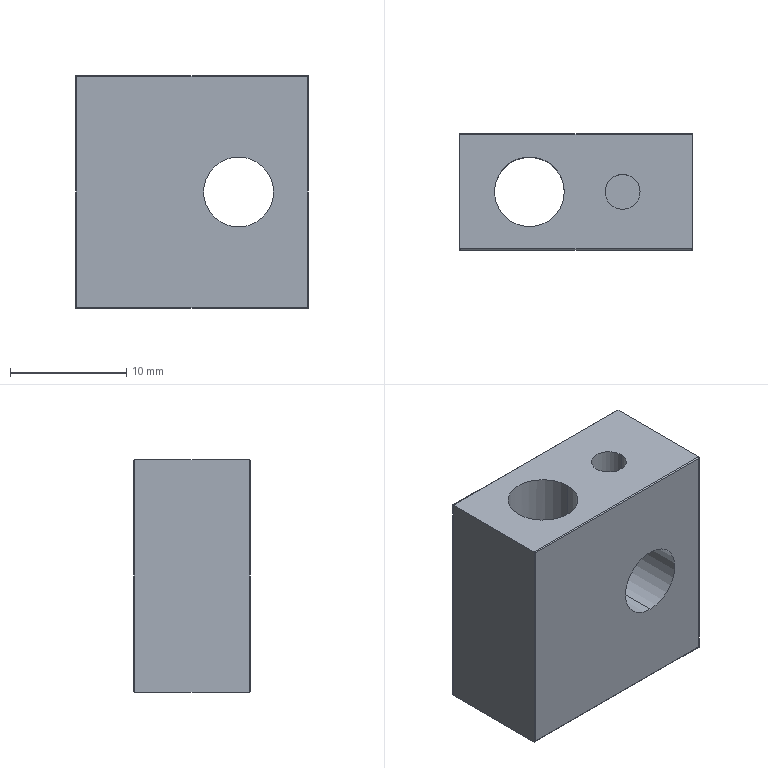Part | SolidWorks | features ICE 3, Extrusion 1, Fillet 1 | 1 solid | 23 faces | box 20 x 10 x 20 mm | volume 3112 mm3 | cylinder 16 | plane 7 | commonest cylinder face diameters 0.2 x8 3 x4 6 x4
STEP:
#1=CARTESIAN_POINT('',(12.5,5.,-3.5));
#2=VERTEX_POINT('',#1);
#3=CARTESIAN_POINT('',(15.5,5.,-3.5));
#4=VERTEX_POINT('',#3);
#5=CARTESIAN_POINT('',(14.,5.,-3.5));
#6=DIRECTION('',(0.,0.,1.));
#7=DIRECTION('',(1.,0.,0.));
#8=AXIS2_PLACEMENT_3D('',#5,#6,#7);
#9=CIRCLE('',#8,1.5);
#10=EDGE_CURVE('',#2,#4,#9,.T.);
#11=ORIENTED_EDGE('',*,*,#10,.F.);
#12=CARTESIAN_POINT('',(12.5,5.,0.));
#13=VERTEX_POINT('',#12);
#14=CARTESIAN_POINT('',(12.5,5.,-3.5));
#15=DIRECTION('',(0.,0.,1.));
#16=VECTOR('',#15,1000.);
#17=LINE('',#14,#16);
#18=EDGE_CURVE('',#2,#13,#17,.T.);
#19=ORIENTED_EDGE('',*,*,#18,.T.);
#20=CARTESIAN_POINT('',(15.5,5.,0.));
#21=VERTEX_POINT('',#20);
#22=CARTESIAN_POINT('',(14.,5.,0.));
#23=DIRECTION('',(0.,0.,1.));
#24=DIRECTION('',(1.,0.,0.));
#25=AXIS2_PLACEMENT_3D('',#22,#23,#24);
#26=CIRCLE('',#25,1.5);
#27=EDGE_CURVE('',#13,#21,#26,.T.);
#28=ORIENTED_EDGE('',*,*,#27,.T.);
#29=CARTESIAN_POINT('',(15.5,5.,-3.5));
#30=DIRECTION('',(0.,0.,1.));
#31=VECTOR('',#30,1000.);
#32=LINE('',#29,#31);
#33=EDGE_CURVE('',#4,#21,#32,.T.);
#34=ORIENTED_EDGE('',*,*,#33,.F.);
#35=EDGE_LOOP('',(#11,#19,#28,#34));
#36=FACE_OUTER_BOUND('',#35,.T.);
#37=CARTESIAN_POINT('',(14.,5.,-3.5));
#38=DIRECTION('',(0.,0.,1.));
#39=DIRECTION('',(1.,0.,0.));
#40=AXIS2_PLACEMENT_3D('',#37,#38,#39);
#41=CYLINDRICAL_SURFACE('',#40,1.5);
#42=ADVANCED_FACE('',(#36),#41,.F.);
#43=CARTESIAN_POINT('',(3.,5.,-20.));
#44=VERTEX_POINT('',#43);
#45=CARTESIAN_POINT('',(9.,5.,-20.));
#46=VERTEX_POINT('',#45);
#47=CARTESIAN_POINT('',(6.,5.,-20.));
#48=DIRECTION('',(0.,0.,1.));
#49=DIRECTION('',(1.,0.,0.));
#50=AXIS2_PLACEMENT_3D('',#47,#48,#49);
#51=CIRCLE('',#50,3.);
#52=EDGE_CURVE('',#44,#46,#51,.T.);
#53=ORIENTED_EDGE('',*,*,#52,.F.);
#54=CARTESIAN_POINT('',(3.,5.,0.));
#55=VERTEX_POINT('',#54);
#56=CARTESIAN_POINT('',(3.,5.,-20.));
#57=DIRECTION('',(0.,0.,1.));
#58=VECTOR('',#57,1000.);
#59=LINE('',#56,#58);
#60=EDGE_CURVE('',#44,#55,#59,.T.);
#61=ORIENTED_EDGE('',*,*,#60,.T.);
#62=CARTESIAN_POINT('',(9.,5.,0.));
#63=VERTEX_POINT('',#62);
#64=CARTESIAN_POINT('',(6.,5.,0.));
#65=DIRECTION('',(0.,0.,1.));
#66=DIRECTION('',(1.,0.,0.));
#67=AXIS2_PLACEMENT_3D('',#64,#65,#66);
#68=CIRCLE('',#67,3.);
#69=EDGE_CURVE('',#55,#63,#68,.T.);
#70=ORIENTED_EDGE('',*,*,#69,.T.);
#71=CARTESIAN_POINT('',(9.,5.,-20.));
#72=DIRECTION('',(0.,0.,1.));
#73=VECTOR('',#72,1000.);
#74=LINE('',#71,#73);
#75=EDGE_CURVE('',#46,#63,#74,.T.);
#76=ORIENTED_EDGE('',*,*,#75,.F.);
#77=EDGE_LOOP('',(#53,#61,#70,#76));
#78=FACE_OUTER_BOUND('',#77,.T.);
#79=CARTESIAN_POINT('',(6.,5.,-20.));
#80=DIRECTION('',(0.,0.,1.));
#81=DIRECTION('',(1.,0.,0.));
#82=AXIS2_PLACEMENT_3D('',#79,#80,#81);
#83=CYLINDRICAL_SURFACE('',#82,3.);
#84=ADVANCED_FACE('',(#78),#83,.F.);
#85=CARTESIAN_POINT('',(6.,8.,-8.5));
#86=VERTEX_POINT('',#85);
#87=CARTESIAN_POINT('',(6.,8.,-11.5));
#88=VERTEX_POINT('',#87);
#89=CARTESIAN_POINT('',(6.,8.,-8.5));
#90=CARTESIAN_POINT('',(5.899,8.,-8.5));
#91=CARTESIAN_POINT('',(5.8,7.995,-8.51));
#92=CARTESIAN_POINT('',(5.606,7.976,-8.549));
#93=CARTESIAN_POINT('',(5.51,7.961,-8.579));
#94=CARTESIAN_POINT('',(5.238,7.907,-8.693));
#95=CARTESIAN_POINT('',(5.074,7.857,-8.804));
#96=CARTESIAN_POINT('',(4.802,7.754,-9.077));
#97=CARTESIAN_POINT('',(4.692,7.701,-9.24));
#98=CARTESIAN_POINT('',(4.579,7.642,-9.51));
#99=CARTESIAN_POINT('',(4.549,7.626,-9.606));
#100=CARTESIAN_POINT('',(4.51,7.604,-9.8));
#101=CARTESIAN_POINT('',(4.5,7.598,-9.899));
#102=CARTESIAN_POINT('',(4.5,7.598,-10.098));
#103=CARTESIAN_POINT('',(4.51,7.604,-10.2));
#104=CARTESIAN_POINT('',(4.549,7.626,-10.394));
#105=CARTESIAN_POINT('',(4.578,7.642,-10.489));
#106=CARTESIAN_POINT('',(4.693,7.702,-10.761));
#107=CARTESIAN_POINT('',(4.803,7.755,-10.924));
#108=CARTESIAN_POINT('',(5.075,7.858,-11.197));
#109=CARTESIAN_POINT('',(5.24,7.908,-11.308));
#110=CARTESIAN_POINT('',(5.6,7.979,-11.459));
#111=CARTESIAN_POINT('',(5.801,8.,-11.5));
#112=CARTESIAN_POINT('',(6.,8.,-11.5));
#113=B_SPLINE_CURVE_WITH_KNOTS('',3,(#89,#90,#91,#92,#93,#94,#95,#96,#97,#98,#99,#100,#101,#102,#103,#104,#105,#106,#107,#108,#109,#110,#111,#112),.UNSPECIFIED.,.F.,.F.,(4,2,2,2,2,2,2,2,2,2,2,4),(0.,0.0002982,0.0005964,0.001193,0.001789,0.002088,0.002386,0.002684,0.002982,0.003579,0.004175,0.004771),.UNSPECIFIED.);
#114=EDGE_CURVE('',#86,#88,#113,.T.);
#115=ORIENTED_EDGE('',*,*,#114,.T.);
#116=CARTESIAN_POINT('',(6.,10.,-11.5));
#117=VERTEX_POINT('',#116);
#118=CARTESIAN_POINT('',(6.,5.,-11.5));
#119=DIRECTION('',(0.,1.,0.));
#120=VECTOR('',#119,1000.);
#121=LINE('',#118,#120);
#122=EDGE_CURVE('',#88,#117,#121,.T.);
#123=ORIENTED_EDGE('',*,*,#122,.T.);
#124=CARTESIAN_POINT('',(6.,10.,-8.5));
#125=VERTEX_POINT('',#124);
#126=CARTESIAN_POINT('',(6.,10.,-10.));
#127=DIRECTION('',(0.,1.,0.));
#128=DIRECTION('',(0.,0.,1.));
#129=AXIS2_PLACEMENT_3D('',#126,#127,#128);
#130=CIRCLE('',#129,1.5);
#131=EDGE_CURVE('',#117,#125,#130,.T.);
#132=ORIENTED_EDGE('',*,*,#131,.T.);
#133=CARTESIAN_POINT('',(6.,5.,-8.5));
#134=DIRECTION('',(0.,1.,0.));
#135=VECTOR('',#134,1000.);
#136=LINE('',#133,#135);
#137=EDGE_CURVE('',#86,#125,#136,.T.);
#138=ORIENTED_EDGE('',*,*,#137,.F.);
#139=EDGE_LOOP('',(#115,#123,#132,#138));
#140=FACE_OUTER_BOUND('',#139,.T.);
#141=CARTESIAN_POINT('',(6.,5.,-10.));
#142=DIRECTION('',(0.,1.,0.));
#143=DIRECTION('',(0.,0.,1.));
#144=AXIS2_PLACEMENT_3D('',#141,#142,#143);
#145=CYLINDRICAL_SURFACE('',#144,1.5);
#146=ADVANCED_FACE('',(#140),#145,.F.);
#147=CARTESIAN_POINT('',(14.,10.,-13.));
#148=VERTEX_POINT('',#147);
#149=CARTESIAN_POINT('',(14.,10.,-7.));
#150=VERTEX_POINT('',#149);
#151=CARTESIAN_POINT('',(14.,10.,-10.));
#152=DIRECTION('',(0.,1.,0.));
#153=DIRECTION('',(0.,0.,1.));
#154=AXIS2_PLACEMENT_3D('',#151,#152,#153);
#155=CIRCLE('',#154,3.);
#156=EDGE_CURVE('',#148,#150,#155,.T.);
#157=ORIENTED_EDGE('',*,*,#156,.T.);
#158=CARTESIAN_POINT('',(14.,0.,-7.));
#159=VERTEX_POINT('',#158);
#160=CARTESIAN_POINT('',(14.,10.,-7.));
#161=DIRECTION('',(0.,-1.,0.));
#162=VECTOR('',#161,1000.);
#163=LINE('',#160,#162);
#164=EDGE_CURVE('',#150,#159,#163,.T.);
#165=ORIENTED_EDGE('',*,*,#164,.T.);
#166=CARTESIAN_POINT('',(14.,0.,-13.));
#167=VERTEX_POINT('',#166);
#168=CARTESIAN_POINT('',(14.,0.,-10.));
#169=DIRECTION('',(0.,1.,0.));
#170=DIRECTION('',(0.,0.,1.));
#171=AXIS2_PLACEMENT_3D('',#168,#169,#170);
#172=CIRCLE('',#171,3.);
#173=EDGE_CURVE('',#167,#159,#172,.T.);
#174=ORIENTED_EDGE('',*,*,#173,.F.);
#175=CARTESIAN_POINT('',(14.,10.,-13.));
#176=DIRECTION('',(0.,-1.,0.));
#177=VECTOR('',#176,1000.);
#178=LINE('',#175,#177);
#179=EDGE_CURVE('',#148,#167,#178,.T.);
#180=ORIENTED_EDGE('',*,*,#179,.F.);
#181=EDGE_LOOP('',(#157,#165,#174,#180));
#182=FACE_OUTER_BOUND('',#181,.T.);
#183=CARTESIAN_POINT('',(14.,10.,-10.));
#184=DIRECTION('',(0.,-1.,0.));
#185=DIRECTION('',(0.,0.,-1.));
#186=AXIS2_PLACEMENT_3D('',#183,#184,#185);
#187=CYLINDRICAL_SURFACE('',#186,3.);
#188=ADVANCED_FACE('',(#182),#187,.F.);
#189=CARTESIAN_POINT('',(14.,5.,0.));
#190=DIRECTION('',(0.,0.,1.));
#191=DIRECTION('',(1.,0.,0.));
#192=AXIS2_PLACEMENT_3D('',#189,#190,#191);
#193=CIRCLE('',#192,1.5);
#194=EDGE_CURVE('',#21,#13,#193,.T.);
#195=ORIENTED_EDGE('',*,*,#194,.F.);
#196=ORIENTED_EDGE('',*,*,#27,.F.);
#197=EDGE_LOOP('',(#195,#196));
#198=FACE_BOUND('',#197,.T.);
#199=CARTESIAN_POINT('',(6.,5.,0.));
#200=DIRECTION('',(0.,0.,1.));
#201=DIRECTION('',(1.,0.,0.));
#202=AXIS2_PLACEMENT_3D('',#199,#200,#201);
#203=CIRCLE('',#202,3.);
#204=EDGE_CURVE('',#63,#55,#203,.T.);
#205=ORIENTED_EDGE('',*,*,#204,.F.);
#206=ORIENTED_EDGE('',*,*,#69,.F.);
#207=EDGE_LOOP('',(#205,#206));
#208=FACE_BOUND('',#207,.T.);
#209=CARTESIAN_POINT('',(0.,9.9,0.));
#210=VERTEX_POINT('',#209);
#211=CARTESIAN_POINT('',(0.,0.1,0.));
#212=VERTEX_POINT('',#211);
#213=CARTESIAN_POINT('',(0.,10.,0.));
#214=DIRECTION('',(0.,-1.,0.));
#215=VECTOR('',#214,1000.);
#216=LINE('',#213,#215);
#217=EDGE_CURVE('',#210,#212,#216,.T.);
#218=ORIENTED_EDGE('',*,*,#217,.T.);
#219=CARTESIAN_POINT('',(20.,0.1,0.));
#220=VERTEX_POINT('',#219);
#221=CARTESIAN_POINT('',(0.,0.1,0.));
#222=DIRECTION('',(1.,0.,0.));
#223=VECTOR('',#222,1000.);
#224=LINE('',#221,#223);
#225=EDGE_CURVE('',#212,#220,#224,.T.);
#226=ORIENTED_EDGE('',*,*,#225,.T.);
#227=CARTESIAN_POINT('',(20.,9.9,0.));
#228=VERTEX_POINT('',#227);
#229=CARTESIAN_POINT('',(20.,10.,0.));
#230=DIRECTION('',(0.,-1.,0.));
#231=VECTOR('',#230,1000.);
#232=LINE('',#229,#231);
#233=EDGE_CURVE('',#228,#220,#232,.T.);
#234=ORIENTED_EDGE('',*,*,#233,.F.);
#235=CARTESIAN_POINT('',(0.,9.9,0.));
#236=DIRECTION('',(-1.,0.,0.));
#237=VECTOR('',#236,1000.);
#238=LINE('',#235,#237);
#239=EDGE_CURVE('',#228,#210,#238,.T.);
#240=ORIENTED_EDGE('',*,*,#239,.T.);
#241=EDGE_LOOP('',(#218,#226,#234,#240));
#242=FACE_OUTER_BOUND('',#241,.T.);
#243=CARTESIAN_POINT('',(0.,10.,0.));
#244=DIRECTION('',(0.,0.,-1.));
#245=DIRECTION('',(-1.,0.,0.));
#246=AXIS2_PLACEMENT_3D('',#243,#244,#245);
#247=PLANE('',#246);
#248=ADVANCED_FACE('',(#198,#208,#242),#247,.F.);
#249=ORIENTED_EDGE('',*,*,#233,.T.);
#250=CARTESIAN_POINT('',(20.,0.1,-20.));
#251=VERTEX_POINT('',#250);
#252=CARTESIAN_POINT('',(20.,0.1,0.));
#253=DIRECTION('',(0.,0.,-1.));
#254=VECTOR('',#253,1000.);
#255=LINE('',#252,#254);
#256=EDGE_CURVE('',#220,#251,#255,.T.);
#257=ORIENTED_EDGE('',*,*,#256,.T.);
#258=CARTESIAN_POINT('',(20.,9.9,-20.));
#259=VERTEX_POINT('',#258);
#260=CARTESIAN_POINT('',(20.,10.,-20.));
#261=DIRECTION('',(0.,-1.,0.));
#262=VECTOR('',#261,1000.);
#263=LINE('',#260,#262);
#264=EDGE_CURVE('',#259,#251,#263,.T.);
#265=ORIENTED_EDGE('',*,*,#264,.F.);
#266=CARTESIAN_POINT('',(20.,9.9,0.));
#267=DIRECTION('',(0.,0.,1.));
#268=VECTOR('',#267,1000.);
#269=LINE('',#266,#268);
#270=EDGE_CURVE('',#259,#228,#269,.T.);
#271=ORIENTED_EDGE('',*,*,#270,.T.);
#272=EDGE_LOOP('',(#249,#257,#265,#271));
#273=FACE_OUTER_BOUND('',#272,.T.);
#274=CARTESIAN_POINT('',(20.,10.,0.));
#275=DIRECTION('',(-1.,0.,0.));
#276=DIRECTION('',(0.,0.,1.));
#277=AXIS2_PLACEMENT_3D('',#274,#275,#276);
#278=PLANE('',#277);
#279=ADVANCED_FACE('',(#273),#278,.F.);
#280=CARTESIAN_POINT('',(6.,5.,-20.));
#281=DIRECTION('',(0.,0.,1.));
#282=DIRECTION('',(1.,0.,0.));
#283=AXIS2_PLACEMENT_3D('',#280,#281,#282);
#284=CIRCLE('',#283,3.);
#285=EDGE_CURVE('',#46,#44,#284,.T.);
#286=ORIENTED_EDGE('',*,*,#285,.T.);
#287=ORIENTED_EDGE('',*,*,#52,.T.);
#288=EDGE_LOOP('',(#286,#287));
#289=FACE_BOUND('',#288,.T.);
#290=ORIENTED_EDGE('',*,*,#264,.T.);
#291=CARTESIAN_POINT('',(0.,0.1,-20.));
#292=VERTEX_POINT('',#291);
#293=CARTESIAN_POINT('',(0.,0.1,-20.));
#294=DIRECTION('',(-1.,0.,0.));
#295=VECTOR('',#294,1000.);
#296=LINE('',#293,#295);
#297=EDGE_CURVE('',#251,#292,#296,.T.);
#298=ORIENTED_EDGE('',*,*,#297,.T.);
#299=CARTESIAN_POINT('',(0.,9.9,-20.));
#300=VERTEX_POINT('',#299);
#301=CARTESIAN_POINT('',(0.,10.,-20.));
#302=DIRECTION('',(0.,-1.,0.));
#303=VECTOR('',#302,1000.);
#304=LINE('',#301,#303);
#305=EDGE_CURVE('',#300,#292,#304,.T.);
#306=ORIENTED_EDGE('',*,*,#305,.F.);
#307=CARTESIAN_POINT('',(0.,9.9,-20.));
#308=DIRECTION('',(1.,0.,0.));
#309=VECTOR('',#308,1000.);
#310=LINE('',#307,#309);
#311=EDGE_CURVE('',#300,#259,#310,.T.);
#312=ORIENTED_EDGE('',*,*,#311,.T.);
#313=EDGE_LOOP('',(#290,#298,#306,#312));
#314=FACE_OUTER_BOUND('',#313,.T.);
#315=CARTESIAN_POINT('',(0.,10.,-20.));
#316=DIRECTION('',(0.,0.,-1.));
#317=DIRECTION('',(-1.,0.,0.));
#318=AXIS2_PLACEMENT_3D('',#315,#316,#317);
#319=PLANE('',#318);
#320=ADVANCED_FACE('',(#289,#314),#319,.T.);
#321=ORIENTED_EDGE('',*,*,#164,.F.);
#322=CARTESIAN_POINT('',(14.,10.,-10.));
#323=DIRECTION('',(0.,1.,0.));
#324=DIRECTION('',(0.,0.,1.));
#325=AXIS2_PLACEMENT_3D('',#322,#323,#324);
#326=CIRCLE('',#325,3.);
#327=EDGE_CURVE('',#150,#148,#326,.T.);
#328=ORIENTED_EDGE('',*,*,#327,.T.);
#329=ORIENTED_EDGE('',*,*,#179,.T.);
#330=CARTESIAN_POINT('',(14.,0.,-10.));
#331=DIRECTION('',(0.,1.,0.));
#332=DIRECTION('',(0.,0.,1.));
#333=AXIS2_PLACEMENT_3D('',#330,#331,#332);
#334=CIRCLE('',#333,3.);
#335=EDGE_CURVE('',#159,#167,#334,.T.);
#336=ORIENTED_EDGE('',*,*,#335,.F.);
#337=EDGE_LOOP('',(#321,#328,#329,#336));
#338=FACE_OUTER_BOUND('',#337,.T.);
#339=CARTESIAN_POINT('',(14.,10.,-10.));
#340=DIRECTION('',(0.,-1.,0.));
#341=DIRECTION('',(0.,0.,-1.));
#342=AXIS2_PLACEMENT_3D('',#339,#340,#341);
#343=CYLINDRICAL_SURFACE('',#342,3.);
#344=ADVANCED_FACE('',(#338),#343,.F.);
#345=ORIENTED_EDGE('',*,*,#305,.T.);
#346=CARTESIAN_POINT('',(0.,0.1,0.));
#347=DIRECTION('',(0.,0.,1.));
#348=VECTOR('',#347,1000.);
#349=LINE('',#346,#348);
#350=EDGE_CURVE('',#292,#212,#349,.T.);
#351=ORIENTED_EDGE('',*,*,#350,.T.);
#352=ORIENTED_EDGE('',*,*,#217,.F.);
#353=CARTESIAN_POINT('',(0.,9.9,0.));
#354=DIRECTION('',(0.,0.,-1.));
#355=VECTOR('',#354,1000.);
#356=LINE('',#353,#355);
#357=EDGE_CURVE('',#210,#300,#356,.T.);
#358=ORIENTED_EDGE('',*,*,#357,.T.);
#359=EDGE_LOOP('',(#345,#351,#352,#358));
#360=FACE_OUTER_BOUND('',#359,.T.);
#361=CARTESIAN_POINT('',(0.,10.,0.));
#362=DIRECTION('',(-1.,0.,0.));
#363=DIRECTION('',(0.,0.,1.));
#364=AXIS2_PLACEMENT_3D('',#361,#362,#363);
#365=PLANE('',#364);
#366=ADVANCED_FACE('',(#360),#365,.T.);
#367=CARTESIAN_POINT('',(19.9,10.,-19.9));
#368=VERTEX_POINT('',#367);
#369=CARTESIAN_POINT('',(0.1,10.,-19.9));
#370=VERTEX_POINT('',#369);
#371=CARTESIAN_POINT('',(0.,10.,-19.9));
#372=DIRECTION('',(-1.,0.,0.));
#373=VECTOR('',#372,1000.);
#374=LINE('',#371,#373);
#375=EDGE_CURVE('',#368,#370,#374,.T.);
#376=ORIENTED_EDGE('',*,*,#375,.T.);
#377=CARTESIAN_POINT('',(0.1,10.,-0.1));
#378=VERTEX_POINT('',#377);
#379=CARTESIAN_POINT('',(0.1,10.,0.));
#380=DIRECTION('',(0.,0.,1.));
#381=VECTOR('',#380,1000.);
#382=LINE('',#379,#381);
#383=EDGE_CURVE('',#370,#378,#382,.T.);
#384=ORIENTED_EDGE('',*,*,#383,.T.);
#385=CARTESIAN_POINT('',(19.9,10.,-0.1));
#386=VERTEX_POINT('',#385);
#387=CARTESIAN_POINT('',(20.,10.,-0.1));
#388=DIRECTION('',(1.,0.,0.));
#389=VECTOR('',#388,1000.);
#390=LINE('',#387,#389);
#391=EDGE_CURVE('',#378,#386,#390,.T.);
#392=ORIENTED_EDGE('',*,*,#391,.T.);
#393=CARTESIAN_POINT('',(19.9,10.,-20.));
#394=DIRECTION('',(0.,0.,-1.));
#395=VECTOR('',#394,1000.);
#396=LINE('',#393,#395);
#397=EDGE_CURVE('',#386,#368,#396,.T.);
#398=ORIENTED_EDGE('',*,*,#397,.T.);
#399=EDGE_LOOP('',(#376,#384,#392,#398));
#400=FACE_OUTER_BOUND('',#399,.T.);
#401=CARTESIAN_POINT('',(6.,10.,-10.));
#402=DIRECTION('',(0.,1.,0.));
#403=DIRECTION('',(0.,0.,1.));
#404=AXIS2_PLACEMENT_3D('',#401,#402,#403);
#405=CIRCLE('',#404,1.5);
#406=EDGE_CURVE('',#125,#117,#405,.T.);
#407=ORIENTED_EDGE('',*,*,#406,.F.);
#408=ORIENTED_EDGE('',*,*,#131,.F.);
#409=EDGE_LOOP('',(#407,#408));
#410=FACE_BOUND('',#409,.T.);
#411=ORIENTED_EDGE('',*,*,#156,.F.);
#412=ORIENTED_EDGE('',*,*,#327,.F.);
#413=EDGE_LOOP('',(#411,#412));
#414=FACE_BOUND('',#413,.T.);
#415=CARTESIAN_POINT('',(0.,10.,0.));
#416=DIRECTION('',(0.,1.,0.));
#417=DIRECTION('',(0.,0.,1.));
#418=AXIS2_PLACEMENT_3D('',#415,#416,#417);
#419=PLANE('',#418);
#420=ADVANCED_FACE('',(#400,#410,#414),#419,.T.);
#421=CARTESIAN_POINT('',(0.1,0.,-19.9));
#422=VERTEX_POINT('',#421);
#423=CARTESIAN_POINT('',(19.9,0.,-19.9));
#424=VERTEX_POINT('',#423);
#425=CARTESIAN_POINT('',(20.,0.,-19.9));
#426=DIRECTION('',(1.,0.,0.));
#427=VECTOR('',#426,1000.);
#428=LINE('',#425,#427);
#429=EDGE_CURVE('',#422,#424,#428,.T.);
#430=ORIENTED_EDGE('',*,*,#429,.T.);
#431=CARTESIAN_POINT('',(19.9,0.,-0.1));
#432=VERTEX_POINT('',#431);
#433=CARTESIAN_POINT('',(19.9,0.,0.));
#434=DIRECTION('',(0.,0.,1.));
#435=VECTOR('',#434,1000.);
#436=LINE('',#433,#435);
#437=EDGE_CURVE('',#424,#432,#436,.T.);
#438=ORIENTED_EDGE('',*,*,#437,.T.);
#439=CARTESIAN_POINT('',(0.1,0.,-0.1));
#440=VERTEX_POINT('',#439);
#441=CARTESIAN_POINT('',(0.,0.,-0.1));
#442=DIRECTION('',(-1.,0.,0.));
#443=VECTOR('',#442,1000.);
#444=LINE('',#441,#443);
#445=EDGE_CURVE('',#432,#440,#444,.T.);
#446=ORIENTED_EDGE('',*,*,#445,.T.);
#447=CARTESIAN_POINT('',(0.1,0.,-20.));
#448=DIRECTION('',(0.,0.,-1.));
#449=VECTOR('',#448,1000.);
#450=LINE('',#447,#449);
#451=EDGE_CURVE('',#440,#422,#450,.T.);
#452=ORIENTED_EDGE('',*,*,#451,.T.);
#453=EDGE_LOOP('',(#430,#438,#446,#452));
#454=FACE_OUTER_BOUND('',#453,.T.);
#455=ORIENTED_EDGE('',*,*,#173,.T.);
#456=ORIENTED_EDGE('',*,*,#335,.T.);
#457=EDGE_LOOP('',(#455,#456));
#458=FACE_BOUND('',#457,.T.);
#459=CARTESIAN_POINT('',(0.,0.,0.));
#460=DIRECTION('',(0.,1.,0.));
#461=DIRECTION('',(0.,0.,1.));
#462=AXIS2_PLACEMENT_3D('',#459,#460,#461);
#463=PLANE('',#462);
#464=ADVANCED_FACE('',(#454,#458),#463,.F.);
#465=ORIENTED_EDGE('',*,*,#122,.F.);
#466=CARTESIAN_POINT('',(6.,8.,-11.5));
#467=CARTESIAN_POINT('',(6.099,8.,-11.5));
#468=CARTESIAN_POINT('',(6.201,7.995,-11.49));
#469=CARTESIAN_POINT('',(6.395,7.975,-11.45));
#470=CARTESIAN_POINT('',(6.489,7.961,-11.421));
#471=CARTESIAN_POINT('',(6.763,7.907,-11.306));
#472=CARTESIAN_POINT('',(6.926,7.857,-11.196));
#473=CARTESIAN_POINT('',(7.13,7.78,-10.991));
#474=CARTESIAN_POINT('',(7.191,7.754,-10.917));
#475=CARTESIAN_POINT('',(7.299,7.705,-10.756));
#476=CARTESIAN_POINT('',(7.346,7.681,-10.669));
#477=CARTESIAN_POINT('',(7.459,7.623,-10.4));
#478=CARTESIAN_POINT('',(7.5,7.598,-10.2));
#479=CARTESIAN_POINT('',(7.5,7.598,-9.902));
#480=CARTESIAN_POINT('',(7.49,7.604,-9.802));
#481=CARTESIAN_POINT('',(7.451,7.626,-9.607));
#482=CARTESIAN_POINT('',(7.422,7.642,-9.513));
#483=CARTESIAN_POINT('',(7.308,7.701,-9.24));
#484=CARTESIAN_POINT('',(7.198,7.754,-9.077));
#485=CARTESIAN_POINT('',(6.993,7.832,-8.872));
#486=CARTESIAN_POINT('',(6.919,7.857,-8.811));
#487=CARTESIAN_POINT('',(6.759,7.904,-8.702));
#488=CARTESIAN_POINT('',(6.671,7.925,-8.655));
#489=CARTESIAN_POINT('',(6.491,7.961,-8.579));
#490=CARTESIAN_POINT('',(6.397,7.975,-8.55));
#491=CARTESIAN_POINT('',(6.202,7.995,-8.51));
#492=CARTESIAN_POINT('',(6.101,8.,-8.5));
#493=CARTESIAN_POINT('',(6.,8.,-8.5));
#494=B_SPLINE_CURVE_WITH_KNOTS('',3,(#466,#467,#468,#469,#470,#471,#472,#473,#474,#475,#476,#477,#478,#479,#480,#481,#482,#483,#484,#485,#486,#487,#488,#489,#490,#491,#492,#493),.UNSPECIFIED.,.F.,.F.,(4,2,2,2,2,2,2,2,2,2,2,2,2,4),(0.004771,0.005069,0.005367,0.005962,0.00626,0.006558,0.007153,0.007451,0.007748,0.008344,0.008642,0.008939,0.009237,0.009535),.UNSPECIFIED.);
#495=EDGE_CURVE('',#88,#86,#494,.T.);
#496=ORIENTED_EDGE('',*,*,#495,.T.);
#497=ORIENTED_EDGE('',*,*,#137,.T.);
#498=ORIENTED_EDGE('',*,*,#406,.T.);
#499=EDGE_LOOP('',(#465,#496,#497,#498));
#500=FACE_OUTER_BOUND('',#499,.T.);
#501=CARTESIAN_POINT('',(6.,5.,-10.));
#502=DIRECTION('',(0.,1.,0.));
#503=DIRECTION('',(0.,0.,1.));
#504=AXIS2_PLACEMENT_3D('',#501,#502,#503);
#505=CYLINDRICAL_SURFACE('',#504,1.5);
#506=ADVANCED_FACE('',(#500),#505,.F.);
#507=ORIENTED_EDGE('',*,*,#60,.F.);
#508=ORIENTED_EDGE('',*,*,#285,.F.);
#509=ORIENTED_EDGE('',*,*,#75,.T.);
#510=ORIENTED_EDGE('',*,*,#204,.T.);
#511=EDGE_LOOP('',(#507,#508,#509,#510));
#512=FACE_OUTER_BOUND('',#511,.T.);
#513=ORIENTED_EDGE('',*,*,#114,.F.);
#514=ORIENTED_EDGE('',*,*,#495,.F.);
#515=EDGE_LOOP('',(#513,#514));
#516=FACE_BOUND('',#515,.T.);
#517=CARTESIAN_POINT('',(6.,5.,-20.));
#518=DIRECTION('',(0.,0.,1.));
#519=DIRECTION('',(1.,0.,0.));
#520=AXIS2_PLACEMENT_3D('',#517,#518,#519);
#521=CYLINDRICAL_SURFACE('',#520,3.);
#522=ADVANCED_FACE('',(#512,#516),#521,.F.);
#523=ORIENTED_EDGE('',*,*,#18,.F.);
#524=CARTESIAN_POINT('',(14.,5.,-3.5));
#525=DIRECTION('',(0.,0.,1.));
#526=DIRECTION('',(1.,0.,0.));
#527=AXIS2_PLACEMENT_3D('',#524,#525,#526);
#528=CIRCLE('',#527,1.5);
#529=EDGE_CURVE('',#4,#2,#528,.T.);
#530=ORIENTED_EDGE('',*,*,#529,.F.);
#531=ORIENTED_EDGE('',*,*,#33,.T.);
#532=ORIENTED_EDGE('',*,*,#194,.T.);
#533=EDGE_LOOP('',(#523,#530,#531,#532));
#534=FACE_OUTER_BOUND('',#533,.T.);
#535=CARTESIAN_POINT('',(14.,5.,-3.5));
#536=DIRECTION('',(0.,0.,1.));
#537=DIRECTION('',(1.,0.,0.));
#538=AXIS2_PLACEMENT_3D('',#535,#536,#537);
#539=CYLINDRICAL_SURFACE('',#538,1.5);
#540=ADVANCED_FACE('',(#534),#539,.F.);
#541=ORIENTED_EDGE('',*,*,#529,.T.);
#542=ORIENTED_EDGE('',*,*,#10,.T.);
#543=EDGE_LOOP('',(#541,#542));
#544=FACE_OUTER_BOUND('',#543,.T.);
#545=CARTESIAN_POINT('',(0.,0.,-3.5));
#546=DIRECTION('',(0.,0.,1.));
#547=DIRECTION('',(1.,0.,0.));
#548=AXIS2_PLACEMENT_3D('',#545,#546,#547);
#549=PLANE('',#548);
#550=ADVANCED_FACE('',(#544),#549,.T.);
#551=CARTESIAN_POINT('',(0.1,0.,-19.9));
#552=CARTESIAN_POINT('',(0.04142,0.,-19.959));
#553=CARTESIAN_POINT('',(0.,0.04142,-20.));
#554=CARTESIAN_POINT('',(0.,0.1,-20.));
#555=(BOUNDED_CURVE()B_SPLINE_CURVE(3,(#551,#552,#553,#554),.UNSPECIFIED.,.F.,.T.)B_SPLINE_CURVE_WITH_KNOTS((4,4),(1.571,3.142),.UNSPECIFIED.)CURVE()GEOMETRIC_REPRESENTATION_ITEM()RATIONAL_B_SPLINE_CURVE((1.,0.8047,0.8047,1.))REPRESENTATION_ITEM(''));
#556=EDGE_CURVE('',#422,#292,#555,.T.);
#557=ORIENTED_EDGE('',*,*,#556,.F.);
#558=ORIENTED_EDGE('',*,*,#451,.F.);
#559=CARTESIAN_POINT('',(0.,0.1,0.));
#560=CARTESIAN_POINT('',(0.,0.04142,0.));
#561=CARTESIAN_POINT('',(0.04142,0.,-0.04142));
#562=CARTESIAN_POINT('',(0.1,0.,-0.1));
#563=(BOUNDED_CURVE()B_SPLINE_CURVE(3,(#559,#560,#561,#562),.UNSPECIFIED.,.F.,.F.)B_SPLINE_CURVE_WITH_KNOTS((4,4),(3.142,4.712),.UNSPECIFIED.)CURVE()GEOMETRIC_REPRESENTATION_ITEM()RATIONAL_B_SPLINE_CURVE((1.,0.8047,0.8047,1.))REPRESENTATION_ITEM(''));
#564=EDGE_CURVE('',#212,#440,#563,.T.);
#565=ORIENTED_EDGE('',*,*,#564,.F.);
#566=ORIENTED_EDGE('',*,*,#350,.F.);
#567=EDGE_LOOP('',(#557,#558,#565,#566));
#568=FACE_OUTER_BOUND('',#567,.T.);
#569=CARTESIAN_POINT('',(0.1,0.1,0.));
#570=DIRECTION('',(0.,0.,1.));
#571=DIRECTION('',(1.,0.,0.));
#572=AXIS2_PLACEMENT_3D('',#569,#570,#571);
#573=CYLINDRICAL_SURFACE('',#572,0.1);
#574=ADVANCED_FACE('',(#568),#573,.T.);
#575=ORIENTED_EDGE('',*,*,#564,.T.);
#576=ORIENTED_EDGE('',*,*,#445,.F.);
#577=CARTESIAN_POINT('',(20.,0.1,0.));
#578=CARTESIAN_POINT('',(20.,0.04142,0.));
#579=CARTESIAN_POINT('',(19.959,0.,-0.04142));
#580=CARTESIAN_POINT('',(19.9,0.,-0.1));
#581=(BOUNDED_CURVE()B_SPLINE_CURVE(3,(#577,#578,#579,#580),.UNSPECIFIED.,.F.,.F.)B_SPLINE_CURVE_WITH_KNOTS((4,4),(0.,1.571),.UNSPECIFIED.)CURVE()GEOMETRIC_REPRESENTATION_ITEM()RATIONAL_B_SPLINE_CURVE((1.,0.8047,0.8047,1.))REPRESENTATION_ITEM(''));
#582=EDGE_CURVE('',#220,#432,#581,.T.);
#583=ORIENTED_EDGE('',*,*,#582,.F.);
#584=ORIENTED_EDGE('',*,*,#225,.F.);
#585=EDGE_LOOP('',(#575,#576,#583,#584));
#586=FACE_OUTER_BOUND('',#585,.T.);
#587=CARTESIAN_POINT('',(0.,0.1,-0.1));
#588=DIRECTION('',(1.,0.,0.));
#589=DIRECTION('',(0.,0.,-1.));
#590=AXIS2_PLACEMENT_3D('',#587,#588,#589);
#591=CYLINDRICAL_SURFACE('',#590,0.1);
#592=ADVANCED_FACE('',(#586),#591,.T.);
#593=ORIENTED_EDGE('',*,*,#556,.T.);
#594=ORIENTED_EDGE('',*,*,#297,.F.);
#595=CARTESIAN_POINT('',(19.9,0.,-19.9));
#596=CARTESIAN_POINT('',(19.959,0.,-19.959));
#597=CARTESIAN_POINT('',(20.,0.04142,-20.));
#598=CARTESIAN_POINT('',(20.,0.1,-20.));
#599=(BOUNDED_CURVE()B_SPLINE_CURVE(3,(#595,#596,#597,#598),.UNSPECIFIED.,.F.,.F.)B_SPLINE_CURVE_WITH_KNOTS((4,4),(1.571,3.142),.UNSPECIFIED.)CURVE()GEOMETRIC_REPRESENTATION_ITEM()RATIONAL_B_SPLINE_CURVE((1.,0.8047,0.8047,1.))REPRESENTATION_ITEM(''));
#600=EDGE_CURVE('',#424,#251,#599,.T.);
#601=ORIENTED_EDGE('',*,*,#600,.F.);
#602=ORIENTED_EDGE('',*,*,#429,.F.);
#603=EDGE_LOOP('',(#593,#594,#601,#602));
#604=FACE_OUTER_BOUND('',#603,.T.);
#605=CARTESIAN_POINT('',(0.,0.1,-19.9));
#606=DIRECTION('',(-1.,0.,0.));
#607=DIRECTION('',(0.,0.,1.));
#608=AXIS2_PLACEMENT_3D('',#605,#606,#607);
#609=CYLINDRICAL_SURFACE('',#608,0.1);
#610=ADVANCED_FACE('',(#604),#609,.T.);
#611=ORIENTED_EDGE('',*,*,#582,.T.);
#612=ORIENTED_EDGE('',*,*,#437,.F.);
#613=ORIENTED_EDGE('',*,*,#600,.T.);
#614=ORIENTED_EDGE('',*,*,#256,.F.);
#615=EDGE_LOOP('',(#611,#612,#613,#614));
#616=FACE_OUTER_BOUND('',#615,.T.);
#617=CARTESIAN_POINT('',(19.9,0.1,0.));
#618=DIRECTION('',(0.,0.,-1.));
#619=DIRECTION('',(-1.,0.,0.));
#620=AXIS2_PLACEMENT_3D('',#617,#618,#619);
#621=CYLINDRICAL_SURFACE('',#620,0.1);
#622=ADVANCED_FACE('',(#616),#621,.T.);
#623=CARTESIAN_POINT('',(19.9,10.,-19.9));
#624=CARTESIAN_POINT('',(19.959,10.,-19.959));
#625=CARTESIAN_POINT('',(20.,9.959,-20.));
#626=CARTESIAN_POINT('',(20.,9.9,-20.));
#627=(BOUNDED_CURVE()B_SPLINE_CURVE(3,(#623,#624,#625,#626),.UNSPECIFIED.,.F.,.T.)B_SPLINE_CURVE_WITH_KNOTS((4,4),(1.571,3.142),.UNSPECIFIED.)CURVE()GEOMETRIC_REPRESENTATION_ITEM()RATIONAL_B_SPLINE_CURVE((1.,0.8047,0.8047,1.))REPRESENTATION_ITEM(''));
#628=EDGE_CURVE('',#368,#259,#627,.T.);
#629=ORIENTED_EDGE('',*,*,#628,.F.);
#630=ORIENTED_EDGE('',*,*,#397,.F.);
#631=CARTESIAN_POINT('',(20.,9.9,0.));
#632=CARTESIAN_POINT('',(20.,9.959,0.));
#633=CARTESIAN_POINT('',(19.959,10.,-0.04142));
#634=CARTESIAN_POINT('',(19.9,10.,-0.1));
#635=(BOUNDED_CURVE()B_SPLINE_CURVE(3,(#631,#632,#633,#634),.UNSPECIFIED.,.F.,.T.)B_SPLINE_CURVE_WITH_KNOTS((4,4),(3.142,4.712),.UNSPECIFIED.)CURVE()GEOMETRIC_REPRESENTATION_ITEM()RATIONAL_B_SPLINE_CURVE((1.,0.8047,0.8047,1.))REPRESENTATION_ITEM(''));
#636=EDGE_CURVE('',#228,#386,#635,.T.);
#637=ORIENTED_EDGE('',*,*,#636,.F.);
#638=ORIENTED_EDGE('',*,*,#270,.F.);
#639=EDGE_LOOP('',(#629,#630,#637,#638));
#640=FACE_OUTER_BOUND('',#639,.T.);
#641=CARTESIAN_POINT('',(19.9,9.9,0.));
#642=DIRECTION('',(0.,0.,1.));
#643=DIRECTION('',(1.,0.,0.));
#644=AXIS2_PLACEMENT_3D('',#641,#642,#643);
#645=CYLINDRICAL_SURFACE('',#644,0.1);
#646=ADVANCED_FACE('',(#640),#645,.T.);
#647=ORIENTED_EDGE('',*,*,#636,.T.);
#648=ORIENTED_EDGE('',*,*,#391,.F.);
#649=CARTESIAN_POINT('',(0.,9.9,0.));
#650=CARTESIAN_POINT('',(0.,9.959,0.));
#651=CARTESIAN_POINT('',(0.04142,10.,-0.04142));
#652=CARTESIAN_POINT('',(0.1,10.,-0.1));
#653=(BOUNDED_CURVE()B_SPLINE_CURVE(3,(#649,#650,#651,#652),.UNSPECIFIED.,.F.,.F.)B_SPLINE_CURVE_WITH_KNOTS((4,4),(0.,1.571),.UNSPECIFIED.)CURVE()GEOMETRIC_REPRESENTATION_ITEM()RATIONAL_B_SPLINE_CURVE((1.,0.8047,0.8047,1.))REPRESENTATION_ITEM(''));
#654=EDGE_CURVE('',#210,#378,#653,.T.);
#655=ORIENTED_EDGE('',*,*,#654,.F.);
#656=ORIENTED_EDGE('',*,*,#239,.F.);
#657=EDGE_LOOP('',(#647,#648,#655,#656));
#658=FACE_OUTER_BOUND('',#657,.T.);
#659=CARTESIAN_POINT('',(0.,9.9,-0.1));
#660=DIRECTION('',(-1.,0.,0.));
#661=DIRECTION('',(0.,0.,1.));
#662=AXIS2_PLACEMENT_3D('',#659,#660,#661);
#663=CYLINDRICAL_SURFACE('',#662,0.1);
#664=ADVANCED_FACE('',(#658),#663,.T.);
#665=ORIENTED_EDGE('',*,*,#628,.T.);
#666=ORIENTED_EDGE('',*,*,#311,.F.);
#667=CARTESIAN_POINT('',(0.1,10.,-19.9));
#668=CARTESIAN_POINT('',(0.04142,10.,-19.959));
#669=CARTESIAN_POINT('',(0.,9.959,-20.));
#670=CARTESIAN_POINT('',(0.,9.9,-20.));
#671=(BOUNDED_CURVE()B_SPLINE_CURVE(3,(#667,#668,#669,#670),.UNSPECIFIED.,.F.,.F.)B_SPLINE_CURVE_WITH_KNOTS((4,4),(1.571,3.142),.UNSPECIFIED.)CURVE()GEOMETRIC_REPRESENTATION_ITEM()RATIONAL_B_SPLINE_CURVE((1.,0.8047,0.8047,1.))REPRESENTATION_ITEM(''));
#672=EDGE_CURVE('',#370,#300,#671,.T.);
#673=ORIENTED_EDGE('',*,*,#672,.F.);
#674=ORIENTED_EDGE('',*,*,#375,.F.);
#675=EDGE_LOOP('',(#665,#666,#673,#674));
#676=FACE_OUTER_BOUND('',#675,.T.);
#677=CARTESIAN_POINT('',(0.,9.9,-19.9));
#678=DIRECTION('',(1.,0.,0.));
#679=DIRECTION('',(0.,0.,-1.));
#680=AXIS2_PLACEMENT_3D('',#677,#678,#679);
#681=CYLINDRICAL_SURFACE('',#680,0.1);
#682=ADVANCED_FACE('',(#676),#681,.T.);
#683=ORIENTED_EDGE('',*,*,#654,.T.);
#684=ORIENTED_EDGE('',*,*,#383,.F.);
#685=ORIENTED_EDGE('',*,*,#672,.T.);
#686=ORIENTED_EDGE('',*,*,#357,.F.);
#687=EDGE_LOOP('',(#683,#684,#685,#686));
#688=FACE_OUTER_BOUND('',#687,.T.);
#689=CARTESIAN_POINT('',(0.1,9.9,0.));
#690=DIRECTION('',(0.,0.,-1.));
#691=DIRECTION('',(-1.,0.,0.));
#692=AXIS2_PLACEMENT_3D('',#689,#690,#691);
#693=CYLINDRICAL_SURFACE('',#692,0.1);
#694=ADVANCED_FACE('',(#688),#693,.T.);
#695=CLOSED_SHELL('',(#42,#84,#146,#188,#248,#279,#320,#344,#366,#420,#464,#506,#522,#540,#550,#574,#592,#610,#622,#646,#664,#682,#694));
#696=MANIFOLD_SOLID_BREP('',#695);
#697=CARTESIAN_POINT('',(0.,0.,0.));
#698=DIRECTION('',(0.,0.,1.));
#699=DIRECTION('',(1.,0.,0.));
#700=AXIS2_PLACEMENT_3D('',#697,#698,#699);
#701=(LENGTH_UNIT()NAMED_UNIT(*)SI_UNIT(.MILLI.,.METRE.));
#702=UNCERTAINTY_MEASURE_WITH_UNIT(LENGTH_MEASURE(0.00001),#701,'','');
#703=(NAMED_UNIT(*)PLANE_ANGLE_UNIT()SI_UNIT($,.RADIAN.));
#704=(NAMED_UNIT(*)SI_UNIT($,.STERADIAN.)SOLID_ANGLE_UNIT());
#705=(GEOMETRIC_REPRESENTATION_CONTEXT(3)GLOBAL_UNCERTAINTY_ASSIGNED_CONTEXT((#702))GLOBAL_UNIT_ASSIGNED_CONTEXT((#701,#703,#704))REPRESENTATION_CONTEXT('',''));
#706=ADVANCED_BREP_SHAPE_REPRESENTATION('',(#696,#700),#705);